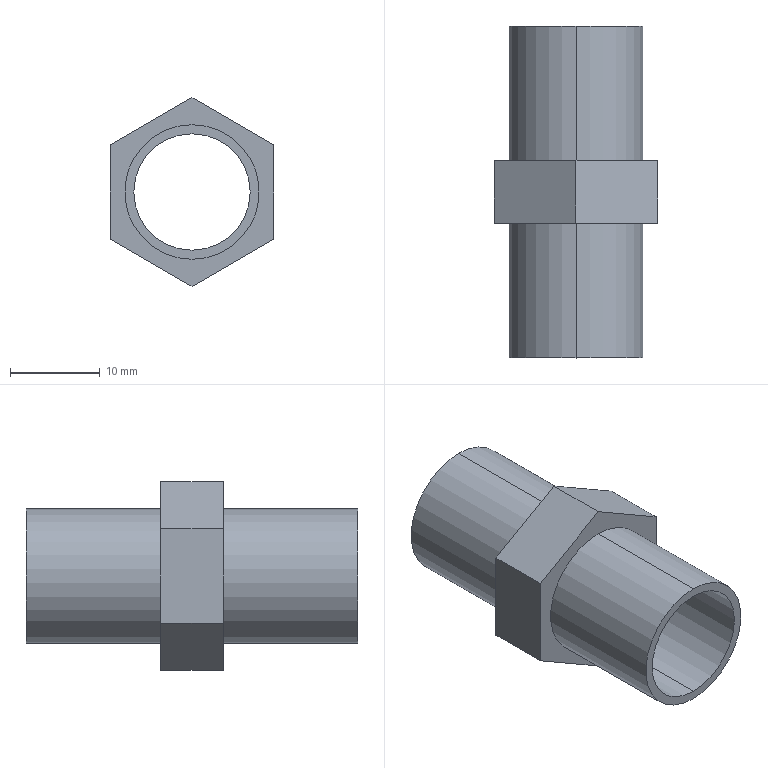Part | SolidWorks | features ICE 3, Extrusion 1 | 1 solid | 16 faces | box 18.246 x 37 x 21.069 mm | volume 2425 mm3 | plane 10 | cylinder 6 | commonest cylinder face diameters 15 x4 12.978 x2
STEP:
#1=CARTESIAN_POINT('',(0.,0.,-6.489));
#2=VERTEX_POINT('',#1);
#3=CARTESIAN_POINT('',(0.,0.,6.489));
#4=VERTEX_POINT('',#3);
#5=CARTESIAN_POINT('',(0.,0.,0.));
#6=DIRECTION('',(0.,1.,0.));
#7=DIRECTION('',(0.,0.,1.));
#8=AXIS2_PLACEMENT_3D('',#5,#6,#7);
#9=CIRCLE('',#8,6.489);
#10=EDGE_CURVE('',#2,#4,#9,.T.);
#11=ORIENTED_EDGE('',*,*,#10,.F.);
#12=CARTESIAN_POINT('',(0.,37.,-6.489));
#13=VERTEX_POINT('',#12);
#14=CARTESIAN_POINT('',(0.,0.,-6.489));
#15=DIRECTION('',(0.,1.,0.));
#16=VECTOR('',#15,1000.);
#17=LINE('',#14,#16);
#18=EDGE_CURVE('',#2,#13,#17,.T.);
#19=ORIENTED_EDGE('',*,*,#18,.T.);
#20=CARTESIAN_POINT('',(0.,37.,6.489));
#21=VERTEX_POINT('',#20);
#22=CARTESIAN_POINT('',(0.,37.,0.));
#23=DIRECTION('',(0.,1.,0.));
#24=DIRECTION('',(0.,0.,1.));
#25=AXIS2_PLACEMENT_3D('',#22,#23,#24);
#26=CIRCLE('',#25,6.489);
#27=EDGE_CURVE('',#13,#21,#26,.T.);
#28=ORIENTED_EDGE('',*,*,#27,.T.);
#29=CARTESIAN_POINT('',(0.,0.,6.489));
#30=DIRECTION('',(0.,1.,0.));
#31=VECTOR('',#30,1000.);
#32=LINE('',#29,#31);
#33=EDGE_CURVE('',#4,#21,#32,.T.);
#34=ORIENTED_EDGE('',*,*,#33,.F.);
#35=EDGE_LOOP('',(#11,#19,#28,#34));
#36=FACE_OUTER_BOUND('',#35,.T.);
#37=CARTESIAN_POINT('',(0.,0.,0.));
#38=DIRECTION('',(0.,1.,0.));
#39=DIRECTION('',(0.,0.,1.));
#40=AXIS2_PLACEMENT_3D('',#37,#38,#39);
#41=CYLINDRICAL_SURFACE('',#40,6.489);
#42=ADVANCED_FACE('',(#36),#41,.F.);
#43=CARTESIAN_POINT('',(0.,37.,7.5));
#44=VERTEX_POINT('',#43);
#45=CARTESIAN_POINT('',(0.,37.,-7.5));
#46=VERTEX_POINT('',#45);
#47=CARTESIAN_POINT('',(0.,37.,0.));
#48=DIRECTION('',(0.,1.,0.));
#49=DIRECTION('',(0.,0.,1.));
#50=AXIS2_PLACEMENT_3D('',#47,#48,#49);
#51=CIRCLE('',#50,7.5);
#52=EDGE_CURVE('',#44,#46,#51,.T.);
#53=ORIENTED_EDGE('',*,*,#52,.F.);
#54=CARTESIAN_POINT('',(0.,22.,7.5));
#55=VERTEX_POINT('',#54);
#56=CARTESIAN_POINT('',(0.,37.,7.5));
#57=DIRECTION('',(0.,-1.,0.));
#58=VECTOR('',#57,1000.);
#59=LINE('',#56,#58);
#60=EDGE_CURVE('',#44,#55,#59,.T.);
#61=ORIENTED_EDGE('',*,*,#60,.T.);
#62=CARTESIAN_POINT('',(0.,22.,-7.5));
#63=VERTEX_POINT('',#62);
#64=CARTESIAN_POINT('',(0.,22.,0.));
#65=DIRECTION('',(0.,1.,0.));
#66=DIRECTION('',(0.,0.,1.));
#67=AXIS2_PLACEMENT_3D('',#64,#65,#66);
#68=CIRCLE('',#67,7.5);
#69=EDGE_CURVE('',#55,#63,#68,.T.);
#70=ORIENTED_EDGE('',*,*,#69,.T.);
#71=CARTESIAN_POINT('',(0.,37.,-7.5));
#72=DIRECTION('',(0.,-1.,0.));
#73=VECTOR('',#72,1000.);
#74=LINE('',#71,#73);
#75=EDGE_CURVE('',#46,#63,#74,.T.);
#76=ORIENTED_EDGE('',*,*,#75,.F.);
#77=EDGE_LOOP('',(#53,#61,#70,#76));
#78=FACE_OUTER_BOUND('',#77,.T.);
#79=CARTESIAN_POINT('',(0.,37.,0.));
#80=DIRECTION('',(0.,-1.,0.));
#81=DIRECTION('',(0.,0.,-1.));
#82=AXIS2_PLACEMENT_3D('',#79,#80,#81);
#83=CYLINDRICAL_SURFACE('',#82,7.5);
#84=ADVANCED_FACE('',(#78),#83,.T.);
#85=CARTESIAN_POINT('',(0.,15.,7.5));
#86=VERTEX_POINT('',#85);
#87=CARTESIAN_POINT('',(0.,15.,-7.5));
#88=VERTEX_POINT('',#87);
#89=CARTESIAN_POINT('',(0.,15.,0.));
#90=DIRECTION('',(0.,1.,0.));
#91=DIRECTION('',(0.,0.,1.));
#92=AXIS2_PLACEMENT_3D('',#89,#90,#91);
#93=CIRCLE('',#92,7.5);
#94=EDGE_CURVE('',#86,#88,#93,.T.);
#95=ORIENTED_EDGE('',*,*,#94,.F.);
#96=CARTESIAN_POINT('',(0.,0.,7.5));
#97=VERTEX_POINT('',#96);
#98=CARTESIAN_POINT('',(0.,15.,7.5));
#99=DIRECTION('',(0.,-1.,0.));
#100=VECTOR('',#99,1000.);
#101=LINE('',#98,#100);
#102=EDGE_CURVE('',#86,#97,#101,.T.);
#103=ORIENTED_EDGE('',*,*,#102,.T.);
#104=CARTESIAN_POINT('',(0.,0.,-7.5));
#105=VERTEX_POINT('',#104);
#106=CARTESIAN_POINT('',(0.,0.,0.));
#107=DIRECTION('',(0.,1.,0.));
#108=DIRECTION('',(0.,0.,1.));
#109=AXIS2_PLACEMENT_3D('',#106,#107,#108);
#110=CIRCLE('',#109,7.5);
#111=EDGE_CURVE('',#97,#105,#110,.T.);
#112=ORIENTED_EDGE('',*,*,#111,.T.);
#113=CARTESIAN_POINT('',(0.,15.,-7.5));
#114=DIRECTION('',(0.,-1.,0.));
#115=VECTOR('',#114,1000.);
#116=LINE('',#113,#115);
#117=EDGE_CURVE('',#88,#105,#116,.T.);
#118=ORIENTED_EDGE('',*,*,#117,.F.);
#119=EDGE_LOOP('',(#95,#103,#112,#118));
#120=FACE_OUTER_BOUND('',#119,.T.);
#121=CARTESIAN_POINT('',(0.,15.,0.));
#122=DIRECTION('',(0.,-1.,0.));
#123=DIRECTION('',(0.,0.,-1.));
#124=AXIS2_PLACEMENT_3D('',#121,#122,#123);
#125=CYLINDRICAL_SURFACE('',#124,7.5);
#126=ADVANCED_FACE('',(#120),#125,.T.);
#127=ORIENTED_EDGE('',*,*,#102,.F.);
#128=CARTESIAN_POINT('',(0.,15.,0.));
#129=DIRECTION('',(0.,1.,0.));
#130=DIRECTION('',(0.,0.,1.));
#131=AXIS2_PLACEMENT_3D('',#128,#129,#130);
#132=CIRCLE('',#131,7.5);
#133=EDGE_CURVE('',#88,#86,#132,.T.);
#134=ORIENTED_EDGE('',*,*,#133,.F.);
#135=ORIENTED_EDGE('',*,*,#117,.T.);
#136=CARTESIAN_POINT('',(0.,0.,0.));
#137=DIRECTION('',(0.,1.,0.));
#138=DIRECTION('',(0.,0.,1.));
#139=AXIS2_PLACEMENT_3D('',#136,#137,#138);
#140=CIRCLE('',#139,7.5);
#141=EDGE_CURVE('',#105,#97,#140,.T.);
#142=ORIENTED_EDGE('',*,*,#141,.T.);
#143=EDGE_LOOP('',(#127,#134,#135,#142));
#144=FACE_OUTER_BOUND('',#143,.T.);
#145=CARTESIAN_POINT('',(0.,15.,0.));
#146=DIRECTION('',(0.,-1.,0.));
#147=DIRECTION('',(0.,0.,-1.));
#148=AXIS2_PLACEMENT_3D('',#145,#146,#147);
#149=CYLINDRICAL_SURFACE('',#148,7.5);
#150=ADVANCED_FACE('',(#144),#149,.T.);
#151=CARTESIAN_POINT('',(0.,0.,0.));
#152=DIRECTION('',(0.,1.,0.));
#153=DIRECTION('',(0.,0.,1.));
#154=AXIS2_PLACEMENT_3D('',#151,#152,#153);
#155=CIRCLE('',#154,6.489);
#156=EDGE_CURVE('',#4,#2,#155,.T.);
#157=ORIENTED_EDGE('',*,*,#156,.T.);
#158=ORIENTED_EDGE('',*,*,#10,.T.);
#159=EDGE_LOOP('',(#157,#158));
#160=FACE_BOUND('',#159,.T.);
#161=ORIENTED_EDGE('',*,*,#141,.F.);
#162=ORIENTED_EDGE('',*,*,#111,.F.);
#163=EDGE_LOOP('',(#161,#162));
#164=FACE_OUTER_BOUND('',#163,.T.);
#165=CARTESIAN_POINT('',(0.,0.,0.));
#166=DIRECTION('',(0.,1.,0.));
#167=DIRECTION('',(0.,0.,1.));
#168=AXIS2_PLACEMENT_3D('',#165,#166,#167);
#169=PLANE('',#168);
#170=ADVANCED_FACE('',(#160,#164),#169,.F.);
#171=CARTESIAN_POINT('',(0.,15.,-10.534));
#172=VERTEX_POINT('',#171);
#173=CARTESIAN_POINT('',(-9.123,15.,-5.267));
#174=VERTEX_POINT('',#173);
#175=CARTESIAN_POINT('',(0.,15.,-10.534));
#176=DIRECTION('',(-0.866,0.,0.5));
#177=VECTOR('',#176,1000.);
#178=LINE('',#175,#177);
#179=EDGE_CURVE('',#172,#174,#178,.T.);
#180=ORIENTED_EDGE('',*,*,#179,.T.);
#181=CARTESIAN_POINT('',(-9.123,22.,-5.267));
#182=VERTEX_POINT('',#181);
#183=CARTESIAN_POINT('',(-9.123,22.,-5.267));
#184=DIRECTION('',(0.,-1.,0.));
#185=VECTOR('',#184,1000.);
#186=LINE('',#183,#185);
#187=EDGE_CURVE('',#182,#174,#186,.T.);
#188=ORIENTED_EDGE('',*,*,#187,.F.);
#189=CARTESIAN_POINT('',(0.,22.,-10.534));
#190=VERTEX_POINT('',#189);
#191=CARTESIAN_POINT('',(0.,22.,-10.534));
#192=DIRECTION('',(-0.866,0.,0.5));
#193=VECTOR('',#192,1000.);
#194=LINE('',#191,#193);
#195=EDGE_CURVE('',#190,#182,#194,.T.);
#196=ORIENTED_EDGE('',*,*,#195,.F.);
#197=CARTESIAN_POINT('',(0.,22.,-10.534));
#198=DIRECTION('',(0.,-1.,0.));
#199=VECTOR('',#198,1000.);
#200=LINE('',#197,#199);
#201=EDGE_CURVE('',#190,#172,#200,.T.);
#202=ORIENTED_EDGE('',*,*,#201,.T.);
#203=EDGE_LOOP('',(#180,#188,#196,#202));
#204=FACE_OUTER_BOUND('',#203,.T.);
#205=CARTESIAN_POINT('',(0.,22.,-10.534));
#206=DIRECTION('',(0.5,0.,0.866));
#207=DIRECTION('',(0.866,0.,-0.5));
#208=AXIS2_PLACEMENT_3D('',#205,#206,#207);
#209=PLANE('',#208);
#210=ADVANCED_FACE('',(#204),#209,.F.);
#211=CARTESIAN_POINT('',(-9.123,15.,5.267));
#212=VERTEX_POINT('',#211);
#213=CARTESIAN_POINT('',(-9.123,15.,-5.267));
#214=DIRECTION('',(0.,0.,1.));
#215=VECTOR('',#214,1000.);
#216=LINE('',#213,#215);
#217=EDGE_CURVE('',#174,#212,#216,.T.);
#218=ORIENTED_EDGE('',*,*,#217,.T.);
#219=CARTESIAN_POINT('',(-9.123,22.,5.267));
#220=VERTEX_POINT('',#219);
#221=CARTESIAN_POINT('',(-9.123,22.,5.267));
#222=DIRECTION('',(0.,-1.,0.));
#223=VECTOR('',#222,1000.);
#224=LINE('',#221,#223);
#225=EDGE_CURVE('',#220,#212,#224,.T.);
#226=ORIENTED_EDGE('',*,*,#225,.F.);
#227=CARTESIAN_POINT('',(-9.123,22.,-5.267));
#228=DIRECTION('',(0.,0.,1.));
#229=VECTOR('',#228,1000.);
#230=LINE('',#227,#229);
#231=EDGE_CURVE('',#182,#220,#230,.T.);
#232=ORIENTED_EDGE('',*,*,#231,.F.);
#233=ORIENTED_EDGE('',*,*,#187,.T.);
#234=EDGE_LOOP('',(#218,#226,#232,#233));
#235=FACE_OUTER_BOUND('',#234,.T.);
#236=CARTESIAN_POINT('',(-9.123,22.,-5.267));
#237=DIRECTION('',(1.,0.,0.));
#238=DIRECTION('',(0.,0.,-1.));
#239=AXIS2_PLACEMENT_3D('',#236,#237,#238);
#240=PLANE('',#239);
#241=ADVANCED_FACE('',(#235),#240,.F.);
#242=CARTESIAN_POINT('',(0.,15.,10.534));
#243=VERTEX_POINT('',#242);
#244=CARTESIAN_POINT('',(-9.123,15.,5.267));
#245=DIRECTION('',(0.866,0.,0.5));
#246=VECTOR('',#245,1000.);
#247=LINE('',#244,#246);
#248=EDGE_CURVE('',#212,#243,#247,.T.);
#249=ORIENTED_EDGE('',*,*,#248,.T.);
#250=CARTESIAN_POINT('',(0.,22.,10.534));
#251=VERTEX_POINT('',#250);
#252=CARTESIAN_POINT('',(0.,22.,10.534));
#253=DIRECTION('',(0.,-1.,0.));
#254=VECTOR('',#253,1000.);
#255=LINE('',#252,#254);
#256=EDGE_CURVE('',#251,#243,#255,.T.);
#257=ORIENTED_EDGE('',*,*,#256,.F.);
#258=CARTESIAN_POINT('',(-9.123,22.,5.267));
#259=DIRECTION('',(0.866,0.,0.5));
#260=VECTOR('',#259,1000.);
#261=LINE('',#258,#260);
#262=EDGE_CURVE('',#220,#251,#261,.T.);
#263=ORIENTED_EDGE('',*,*,#262,.F.);
#264=ORIENTED_EDGE('',*,*,#225,.T.);
#265=EDGE_LOOP('',(#249,#257,#263,#264));
#266=FACE_OUTER_BOUND('',#265,.T.);
#267=CARTESIAN_POINT('',(-9.123,22.,5.267));
#268=DIRECTION('',(0.5,0.,-0.866));
#269=DIRECTION('',(-0.866,0.,-0.5));
#270=AXIS2_PLACEMENT_3D('',#267,#268,#269);
#271=PLANE('',#270);
#272=ADVANCED_FACE('',(#266),#271,.F.);
#273=CARTESIAN_POINT('',(9.123,15.,5.267));
#274=VERTEX_POINT('',#273);
#275=CARTESIAN_POINT('',(0.,15.,10.534));
#276=DIRECTION('',(0.866,0.,-0.5));
#277=VECTOR('',#276,1000.);
#278=LINE('',#275,#277);
#279=EDGE_CURVE('',#243,#274,#278,.T.);
#280=ORIENTED_EDGE('',*,*,#279,.T.);
#281=CARTESIAN_POINT('',(9.123,22.,5.267));
#282=VERTEX_POINT('',#281);
#283=CARTESIAN_POINT('',(9.123,22.,5.267));
#284=DIRECTION('',(0.,-1.,0.));
#285=VECTOR('',#284,1000.);
#286=LINE('',#283,#285);
#287=EDGE_CURVE('',#282,#274,#286,.T.);
#288=ORIENTED_EDGE('',*,*,#287,.F.);
#289=CARTESIAN_POINT('',(0.,22.,10.534));
#290=DIRECTION('',(0.866,0.,-0.5));
#291=VECTOR('',#290,1000.);
#292=LINE('',#289,#291);
#293=EDGE_CURVE('',#251,#282,#292,.T.);
#294=ORIENTED_EDGE('',*,*,#293,.F.);
#295=ORIENTED_EDGE('',*,*,#256,.T.);
#296=EDGE_LOOP('',(#280,#288,#294,#295));
#297=FACE_OUTER_BOUND('',#296,.T.);
#298=CARTESIAN_POINT('',(0.,22.,10.534));
#299=DIRECTION('',(-0.5,0.,-0.866));
#300=DIRECTION('',(-0.866,0.,0.5));
#301=AXIS2_PLACEMENT_3D('',#298,#299,#300);
#302=PLANE('',#301);
#303=ADVANCED_FACE('',(#297),#302,.F.);
#304=CARTESIAN_POINT('',(9.123,15.,-5.267));
#305=VERTEX_POINT('',#304);
#306=CARTESIAN_POINT('',(9.123,15.,5.267));
#307=DIRECTION('',(0.,0.,-1.));
#308=VECTOR('',#307,1000.);
#309=LINE('',#306,#308);
#310=EDGE_CURVE('',#274,#305,#309,.T.);
#311=ORIENTED_EDGE('',*,*,#310,.T.);
#312=CARTESIAN_POINT('',(9.123,22.,-5.267));
#313=VERTEX_POINT('',#312);
#314=CARTESIAN_POINT('',(9.123,22.,-5.267));
#315=DIRECTION('',(0.,-1.,0.));
#316=VECTOR('',#315,1000.);
#317=LINE('',#314,#316);
#318=EDGE_CURVE('',#313,#305,#317,.T.);
#319=ORIENTED_EDGE('',*,*,#318,.F.);
#320=CARTESIAN_POINT('',(9.123,22.,5.267));
#321=DIRECTION('',(0.,0.,-1.));
#322=VECTOR('',#321,1000.);
#323=LINE('',#320,#322);
#324=EDGE_CURVE('',#282,#313,#323,.T.);
#325=ORIENTED_EDGE('',*,*,#324,.F.);
#326=ORIENTED_EDGE('',*,*,#287,.T.);
#327=EDGE_LOOP('',(#311,#319,#325,#326));
#328=FACE_OUTER_BOUND('',#327,.T.);
#329=CARTESIAN_POINT('',(9.123,22.,5.267));
#330=DIRECTION('',(-1.,0.,0.));
#331=DIRECTION('',(0.,0.,1.));
#332=AXIS2_PLACEMENT_3D('',#329,#330,#331);
#333=PLANE('',#332);
#334=ADVANCED_FACE('',(#328),#333,.F.);
#335=CARTESIAN_POINT('',(9.123,15.,-5.267));
#336=DIRECTION('',(-0.866,0.,-0.5));
#337=VECTOR('',#336,1000.);
#338=LINE('',#335,#337);
#339=EDGE_CURVE('',#305,#172,#338,.T.);
#340=ORIENTED_EDGE('',*,*,#339,.T.);
#341=ORIENTED_EDGE('',*,*,#201,.F.);
#342=CARTESIAN_POINT('',(9.123,22.,-5.267));
#343=DIRECTION('',(-0.866,0.,-0.5));
#344=VECTOR('',#343,1000.);
#345=LINE('',#342,#344);
#346=EDGE_CURVE('',#313,#190,#345,.T.);
#347=ORIENTED_EDGE('',*,*,#346,.F.);
#348=ORIENTED_EDGE('',*,*,#318,.T.);
#349=EDGE_LOOP('',(#340,#341,#347,#348));
#350=FACE_OUTER_BOUND('',#349,.T.);
#351=CARTESIAN_POINT('',(9.123,22.,-5.267));
#352=DIRECTION('',(-0.5,0.,0.866));
#353=DIRECTION('',(0.866,0.,0.5));
#354=AXIS2_PLACEMENT_3D('',#351,#352,#353);
#355=PLANE('',#354);
#356=ADVANCED_FACE('',(#350),#355,.F.);
#357=CARTESIAN_POINT('',(0.,22.,0.));
#358=DIRECTION('',(0.,1.,0.));
#359=DIRECTION('',(0.,0.,1.));
#360=AXIS2_PLACEMENT_3D('',#357,#358,#359);
#361=CIRCLE('',#360,7.5);
#362=EDGE_CURVE('',#63,#55,#361,.T.);
#363=ORIENTED_EDGE('',*,*,#362,.F.);
#364=ORIENTED_EDGE('',*,*,#69,.F.);
#365=EDGE_LOOP('',(#363,#364));
#366=FACE_BOUND('',#365,.T.);
#367=ORIENTED_EDGE('',*,*,#195,.T.);
#368=ORIENTED_EDGE('',*,*,#231,.T.);
#369=ORIENTED_EDGE('',*,*,#262,.T.);
#370=ORIENTED_EDGE('',*,*,#293,.T.);
#371=ORIENTED_EDGE('',*,*,#324,.T.);
#372=ORIENTED_EDGE('',*,*,#346,.T.);
#373=EDGE_LOOP('',(#367,#368,#369,#370,#371,#372));
#374=FACE_OUTER_BOUND('',#373,.T.);
#375=CARTESIAN_POINT('',(0.,22.,0.));
#376=DIRECTION('',(0.,1.,0.));
#377=DIRECTION('',(0.,0.,1.));
#378=AXIS2_PLACEMENT_3D('',#375,#376,#377);
#379=PLANE('',#378);
#380=ADVANCED_FACE('',(#366,#374),#379,.T.);
#381=ORIENTED_EDGE('',*,*,#133,.T.);
#382=ORIENTED_EDGE('',*,*,#94,.T.);
#383=EDGE_LOOP('',(#381,#382));
#384=FACE_BOUND('',#383,.T.);
#385=ORIENTED_EDGE('',*,*,#179,.F.);
#386=ORIENTED_EDGE('',*,*,#339,.F.);
#387=ORIENTED_EDGE('',*,*,#310,.F.);
#388=ORIENTED_EDGE('',*,*,#279,.F.);
#389=ORIENTED_EDGE('',*,*,#248,.F.);
#390=ORIENTED_EDGE('',*,*,#217,.F.);
#391=EDGE_LOOP('',(#385,#386,#387,#388,#389,#390));
#392=FACE_OUTER_BOUND('',#391,.T.);
#393=CARTESIAN_POINT('',(0.,15.,0.));
#394=DIRECTION('',(0.,1.,0.));
#395=DIRECTION('',(0.,0.,1.));
#396=AXIS2_PLACEMENT_3D('',#393,#394,#395);
#397=PLANE('',#396);
#398=ADVANCED_FACE('',(#384,#392),#397,.F.);
#399=ORIENTED_EDGE('',*,*,#60,.F.);
#400=CARTESIAN_POINT('',(0.,37.,0.));
#401=DIRECTION('',(0.,1.,0.));
#402=DIRECTION('',(0.,0.,1.));
#403=AXIS2_PLACEMENT_3D('',#400,#401,#402);
#404=CIRCLE('',#403,7.5);
#405=EDGE_CURVE('',#46,#44,#404,.T.);
#406=ORIENTED_EDGE('',*,*,#405,.F.);
#407=ORIENTED_EDGE('',*,*,#75,.T.);
#408=ORIENTED_EDGE('',*,*,#362,.T.);
#409=EDGE_LOOP('',(#399,#406,#407,#408));
#410=FACE_OUTER_BOUND('',#409,.T.);
#411=CARTESIAN_POINT('',(0.,37.,0.));
#412=DIRECTION('',(0.,-1.,0.));
#413=DIRECTION('',(0.,0.,-1.));
#414=AXIS2_PLACEMENT_3D('',#411,#412,#413);
#415=CYLINDRICAL_SURFACE('',#414,7.5);
#416=ADVANCED_FACE('',(#410),#415,.T.);
#417=CARTESIAN_POINT('',(0.,37.,0.));
#418=DIRECTION('',(0.,1.,0.));
#419=DIRECTION('',(0.,0.,1.));
#420=AXIS2_PLACEMENT_3D('',#417,#418,#419);
#421=CIRCLE('',#420,6.489);
#422=EDGE_CURVE('',#21,#13,#421,.T.);
#423=ORIENTED_EDGE('',*,*,#422,.F.);
#424=ORIENTED_EDGE('',*,*,#27,.F.);
#425=EDGE_LOOP('',(#423,#424));
#426=FACE_BOUND('',#425,.T.);
#427=ORIENTED_EDGE('',*,*,#405,.T.);
#428=ORIENTED_EDGE('',*,*,#52,.T.);
#429=EDGE_LOOP('',(#427,#428));
#430=FACE_OUTER_BOUND('',#429,.T.);
#431=CARTESIAN_POINT('',(0.,37.,0.));
#432=DIRECTION('',(0.,1.,0.));
#433=DIRECTION('',(0.,0.,1.));
#434=AXIS2_PLACEMENT_3D('',#431,#432,#433);
#435=PLANE('',#434);
#436=ADVANCED_FACE('',(#426,#430),#435,.T.);
#437=ORIENTED_EDGE('',*,*,#18,.F.);
#438=ORIENTED_EDGE('',*,*,#156,.F.);
#439=ORIENTED_EDGE('',*,*,#33,.T.);
#440=ORIENTED_EDGE('',*,*,#422,.T.);
#441=EDGE_LOOP('',(#437,#438,#439,#440));
#442=FACE_OUTER_BOUND('',#441,.T.);
#443=CARTESIAN_POINT('',(0.,0.,0.));
#444=DIRECTION('',(0.,1.,0.));
#445=DIRECTION('',(0.,0.,1.));
#446=AXIS2_PLACEMENT_3D('',#443,#444,#445);
#447=CYLINDRICAL_SURFACE('',#446,6.489);
#448=ADVANCED_FACE('',(#442),#447,.F.);
#449=CLOSED_SHELL('',(#42,#84,#126,#150,#170,#210,#241,#272,#303,#334,#356,#380,#398,#416,#436,#448));
#450=MANIFOLD_SOLID_BREP('',#449);
#451=CARTESIAN_POINT('',(0.,0.,0.));
#452=DIRECTION('',(0.,0.,1.));
#453=DIRECTION('',(1.,0.,0.));
#454=AXIS2_PLACEMENT_3D('',#451,#452,#453);
#455=(LENGTH_UNIT()NAMED_UNIT(*)SI_UNIT(.MILLI.,.METRE.));
#456=UNCERTAINTY_MEASURE_WITH_UNIT(LENGTH_MEASURE(0.00001),#455,'','');
#457=(NAMED_UNIT(*)PLANE_ANGLE_UNIT()SI_UNIT($,.RADIAN.));
#458=(NAMED_UNIT(*)SI_UNIT($,.STERADIAN.)SOLID_ANGLE_UNIT());
#459=(GEOMETRIC_REPRESENTATION_CONTEXT(3)GLOBAL_UNCERTAINTY_ASSIGNED_CONTEXT((#456))GLOBAL_UNIT_ASSIGNED_CONTEXT((#455,#457,#458))REPRESENTATION_CONTEXT('',''));
#460=ADVANCED_BREP_SHAPE_REPRESENTATION('',(#450,#454),#459);